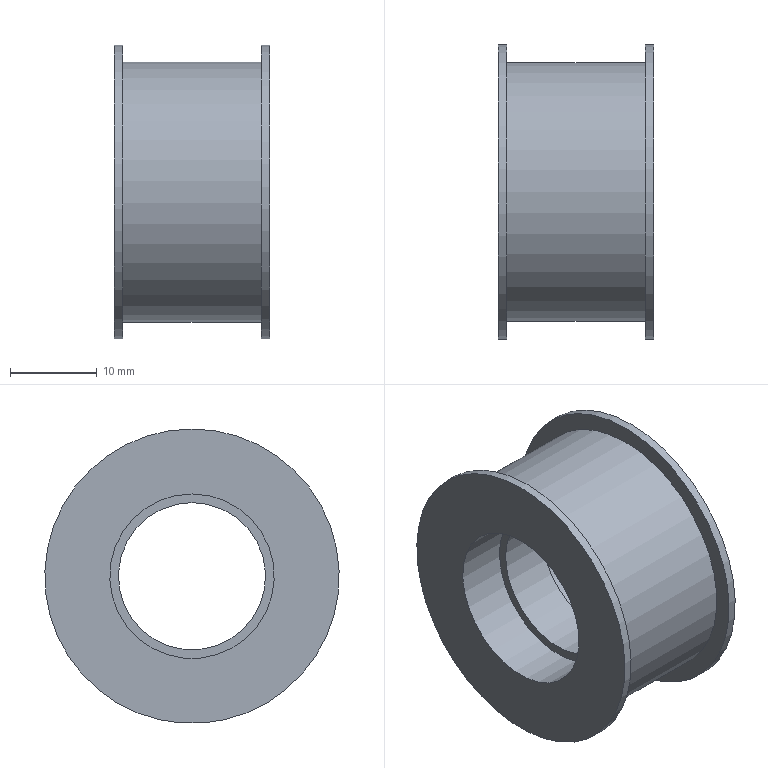Part | NX | 1 solid | 12 faces | box 18 x 34 x 34 mm | volume 8361 mm3 | cylinder 6 | plane 6 | commonest cylinder face diameters 19 x2 34 x2 17 x1 30 x1
STEP:
#1=CARTESIAN_POINT('',(-9.,0.,17.));
#2=VERTEX_POINT('',#1);
#3=CARTESIAN_POINT('',(-9.,0.,0.));
#4=DIRECTION('',(-1.,0.,0.));
#5=DIRECTION('',(0.,0.,1.));
#6=AXIS2_PLACEMENT_3D('',#3,#4,#5);
#7=CIRCLE('',#6,17.);
#8=EDGE_CURVE('',#2,#2,#7,.T.);
#9=ORIENTED_EDGE('',*,*,#8,.F.);
#10=EDGE_LOOP('',(#9));
#11=FACE_BOUND('',#10,.T.);
#12=CARTESIAN_POINT('',(-8.,0.,17.));
#13=VERTEX_POINT('',#12);
#14=CARTESIAN_POINT('',(-8.,0.,0.));
#15=DIRECTION('',(-1.,0.,0.));
#16=DIRECTION('',(0.,0.,1.));
#17=AXIS2_PLACEMENT_3D('',#14,#15,#16);
#18=CIRCLE('',#17,17.);
#19=EDGE_CURVE('',#13,#13,#18,.T.);
#20=ORIENTED_EDGE('',*,*,#19,.T.);
#21=EDGE_LOOP('',(#20));
#22=FACE_BOUND('',#21,.T.);
#23=CARTESIAN_POINT('',(9.,0.,0.));
#24=DIRECTION('',(-1.,0.,0.));
#25=DIRECTION('',(0.,0.,1.));
#26=AXIS2_PLACEMENT_3D('',#23,#24,#25);
#27=CYLINDRICAL_SURFACE('',#26,17.);
#28=ADVANCED_FACE('',(#11,#22),#27,.T.);
#29=CARTESIAN_POINT('',(-9.,0.,9.5));
#30=VERTEX_POINT('',#29);
#31=CARTESIAN_POINT('',(-9.,0.,0.));
#32=DIRECTION('',(-1.,0.,0.));
#33=DIRECTION('',(0.,0.,1.));
#34=AXIS2_PLACEMENT_3D('',#31,#32,#33);
#35=CIRCLE('',#34,9.5);
#36=EDGE_CURVE('',#30,#30,#35,.T.);
#37=ORIENTED_EDGE('',*,*,#36,.F.);
#38=EDGE_LOOP('',(#37));
#39=FACE_BOUND('',#38,.T.);
#40=ORIENTED_EDGE('',*,*,#8,.T.);
#41=EDGE_LOOP('',(#40));
#42=FACE_BOUND('',#41,.T.);
#43=CARTESIAN_POINT('',(-9.,17.,0.));
#44=DIRECTION('',(1.,0.,0.));
#45=DIRECTION('',(0.,0.,-1.));
#46=AXIS2_PLACEMENT_3D('',#43,#44,#45);
#47=PLANE('',#46);
#48=ADVANCED_FACE('',(#39,#42),#47,.F.);
#49=CARTESIAN_POINT('',(-3.,0.,9.5));
#50=VERTEX_POINT('',#49);
#51=CARTESIAN_POINT('',(-3.,0.,0.));
#52=DIRECTION('',(-1.,0.,0.));
#53=DIRECTION('',(0.,0.,1.));
#54=AXIS2_PLACEMENT_3D('',#51,#52,#53);
#55=CIRCLE('',#54,9.5);
#56=EDGE_CURVE('',#50,#50,#55,.T.);
#57=ORIENTED_EDGE('',*,*,#56,.F.);
#58=EDGE_LOOP('',(#57));
#59=FACE_BOUND('',#58,.T.);
#60=ORIENTED_EDGE('',*,*,#36,.T.);
#61=EDGE_LOOP('',(#60));
#62=FACE_BOUND('',#61,.T.);
#63=CARTESIAN_POINT('',(9.,0.,0.));
#64=DIRECTION('',(-1.,0.,0.));
#65=DIRECTION('',(0.,0.,1.));
#66=AXIS2_PLACEMENT_3D('',#63,#64,#65);
#67=CYLINDRICAL_SURFACE('',#66,9.5);
#68=ADVANCED_FACE('',(#59,#62),#67,.F.);
#69=CARTESIAN_POINT('',(-3.,0.,8.5));
#70=VERTEX_POINT('',#69);
#71=CARTESIAN_POINT('',(-3.,0.,0.));
#72=DIRECTION('',(-1.,0.,0.));
#73=DIRECTION('',(0.,0.,1.));
#74=AXIS2_PLACEMENT_3D('',#71,#72,#73);
#75=CIRCLE('',#74,8.5);
#76=EDGE_CURVE('',#70,#70,#75,.T.);
#77=ORIENTED_EDGE('',*,*,#76,.F.);
#78=EDGE_LOOP('',(#77));
#79=FACE_BOUND('',#78,.T.);
#80=ORIENTED_EDGE('',*,*,#56,.T.);
#81=EDGE_LOOP('',(#80));
#82=FACE_BOUND('',#81,.T.);
#83=CARTESIAN_POINT('',(-3.,9.5,0.));
#84=DIRECTION('',(1.,0.,0.));
#85=DIRECTION('',(0.,0.,-1.));
#86=AXIS2_PLACEMENT_3D('',#83,#84,#85);
#87=PLANE('',#86);
#88=ADVANCED_FACE('',(#79,#82),#87,.F.);
#89=CARTESIAN_POINT('',(3.,0.,8.5));
#90=VERTEX_POINT('',#89);
#91=CARTESIAN_POINT('',(3.,0.,0.));
#92=DIRECTION('',(-1.,0.,0.));
#93=DIRECTION('',(0.,0.,1.));
#94=AXIS2_PLACEMENT_3D('',#91,#92,#93);
#95=CIRCLE('',#94,8.5);
#96=EDGE_CURVE('',#90,#90,#95,.T.);
#97=ORIENTED_EDGE('',*,*,#96,.F.);
#98=EDGE_LOOP('',(#97));
#99=FACE_BOUND('',#98,.T.);
#100=ORIENTED_EDGE('',*,*,#76,.T.);
#101=EDGE_LOOP('',(#100));
#102=FACE_BOUND('',#101,.T.);
#103=CARTESIAN_POINT('',(9.,0.,0.));
#104=DIRECTION('',(-1.,0.,0.));
#105=DIRECTION('',(0.,0.,1.));
#106=AXIS2_PLACEMENT_3D('',#103,#104,#105);
#107=CYLINDRICAL_SURFACE('',#106,8.5);
#108=ADVANCED_FACE('',(#99,#102),#107,.F.);
#109=CARTESIAN_POINT('',(3.,0.,9.5));
#110=VERTEX_POINT('',#109);
#111=CARTESIAN_POINT('',(3.,0.,0.));
#112=DIRECTION('',(-1.,0.,0.));
#113=DIRECTION('',(0.,0.,1.));
#114=AXIS2_PLACEMENT_3D('',#111,#112,#113);
#115=CIRCLE('',#114,9.5);
#116=EDGE_CURVE('',#110,#110,#115,.T.);
#117=ORIENTED_EDGE('',*,*,#116,.F.);
#118=EDGE_LOOP('',(#117));
#119=FACE_BOUND('',#118,.T.);
#120=ORIENTED_EDGE('',*,*,#96,.T.);
#121=EDGE_LOOP('',(#120));
#122=FACE_BOUND('',#121,.T.);
#123=CARTESIAN_POINT('',(3.,8.5,0.));
#124=DIRECTION('',(-1.,0.,0.));
#125=DIRECTION('',(0.,0.,1.));
#126=AXIS2_PLACEMENT_3D('',#123,#124,#125);
#127=PLANE('',#126);
#128=ADVANCED_FACE('',(#119,#122),#127,.F.);
#129=CARTESIAN_POINT('',(9.,0.,9.5));
#130=VERTEX_POINT('',#129);
#131=CARTESIAN_POINT('',(9.,0.,0.));
#132=DIRECTION('',(-1.,0.,0.));
#133=DIRECTION('',(0.,0.,1.));
#134=AXIS2_PLACEMENT_3D('',#131,#132,#133);
#135=CIRCLE('',#134,9.5);
#136=EDGE_CURVE('',#130,#130,#135,.T.);
#137=ORIENTED_EDGE('',*,*,#136,.F.);
#138=EDGE_LOOP('',(#137));
#139=FACE_BOUND('',#138,.T.);
#140=ORIENTED_EDGE('',*,*,#116,.T.);
#141=EDGE_LOOP('',(#140));
#142=FACE_BOUND('',#141,.T.);
#143=CARTESIAN_POINT('',(9.,0.,0.));
#144=DIRECTION('',(-1.,0.,0.));
#145=DIRECTION('',(0.,0.,1.));
#146=AXIS2_PLACEMENT_3D('',#143,#144,#145);
#147=CYLINDRICAL_SURFACE('',#146,9.5);
#148=ADVANCED_FACE('',(#139,#142),#147,.F.);
#149=CARTESIAN_POINT('',(9.,0.,17.));
#150=VERTEX_POINT('',#149);
#151=CARTESIAN_POINT('',(9.,0.,0.));
#152=DIRECTION('',(-1.,0.,0.));
#153=DIRECTION('',(0.,0.,1.));
#154=AXIS2_PLACEMENT_3D('',#151,#152,#153);
#155=CIRCLE('',#154,17.);
#156=EDGE_CURVE('',#150,#150,#155,.T.);
#157=ORIENTED_EDGE('',*,*,#156,.F.);
#158=EDGE_LOOP('',(#157));
#159=FACE_BOUND('',#158,.T.);
#160=ORIENTED_EDGE('',*,*,#136,.T.);
#161=EDGE_LOOP('',(#160));
#162=FACE_BOUND('',#161,.T.);
#163=CARTESIAN_POINT('',(9.,9.5,0.));
#164=DIRECTION('',(-1.,0.,0.));
#165=DIRECTION('',(0.,0.,1.));
#166=AXIS2_PLACEMENT_3D('',#163,#164,#165);
#167=PLANE('',#166);
#168=ADVANCED_FACE('',(#159,#162),#167,.F.);
#169=CARTESIAN_POINT('',(8.,0.,17.));
#170=VERTEX_POINT('',#169);
#171=CARTESIAN_POINT('',(8.,0.,0.));
#172=DIRECTION('',(-1.,0.,0.));
#173=DIRECTION('',(0.,0.,1.));
#174=AXIS2_PLACEMENT_3D('',#171,#172,#173);
#175=CIRCLE('',#174,17.);
#176=EDGE_CURVE('',#170,#170,#175,.T.);
#177=ORIENTED_EDGE('',*,*,#176,.F.);
#178=EDGE_LOOP('',(#177));
#179=FACE_BOUND('',#178,.T.);
#180=ORIENTED_EDGE('',*,*,#156,.T.);
#181=EDGE_LOOP('',(#180));
#182=FACE_BOUND('',#181,.T.);
#183=CARTESIAN_POINT('',(9.,0.,0.));
#184=DIRECTION('',(-1.,0.,0.));
#185=DIRECTION('',(0.,0.,1.));
#186=AXIS2_PLACEMENT_3D('',#183,#184,#185);
#187=CYLINDRICAL_SURFACE('',#186,17.);
#188=ADVANCED_FACE('',(#179,#182),#187,.T.);
#189=CARTESIAN_POINT('',(8.,0.,15.));
#190=VERTEX_POINT('',#189);
#191=CARTESIAN_POINT('',(8.,0.,0.));
#192=DIRECTION('',(-1.,0.,0.));
#193=DIRECTION('',(0.,0.,1.));
#194=AXIS2_PLACEMENT_3D('',#191,#192,#193);
#195=CIRCLE('',#194,15.);
#196=EDGE_CURVE('',#190,#190,#195,.T.);
#197=ORIENTED_EDGE('',*,*,#196,.F.);
#198=EDGE_LOOP('',(#197));
#199=FACE_BOUND('',#198,.T.);
#200=ORIENTED_EDGE('',*,*,#176,.T.);
#201=EDGE_LOOP('',(#200));
#202=FACE_BOUND('',#201,.T.);
#203=CARTESIAN_POINT('',(8.,17.,0.));
#204=DIRECTION('',(1.,0.,0.));
#205=DIRECTION('',(0.,0.,-1.));
#206=AXIS2_PLACEMENT_3D('',#203,#204,#205);
#207=PLANE('',#206);
#208=ADVANCED_FACE('',(#199,#202),#207,.F.);
#209=CARTESIAN_POINT('',(-8.,0.,15.));
#210=VERTEX_POINT('',#209);
#211=CARTESIAN_POINT('',(-8.,0.,0.));
#212=DIRECTION('',(-1.,0.,0.));
#213=DIRECTION('',(0.,0.,1.));
#214=AXIS2_PLACEMENT_3D('',#211,#212,#213);
#215=CIRCLE('',#214,15.);
#216=EDGE_CURVE('',#210,#210,#215,.T.);
#217=ORIENTED_EDGE('',*,*,#216,.F.);
#218=EDGE_LOOP('',(#217));
#219=FACE_BOUND('',#218,.T.);
#220=ORIENTED_EDGE('',*,*,#196,.T.);
#221=EDGE_LOOP('',(#220));
#222=FACE_BOUND('',#221,.T.);
#223=CARTESIAN_POINT('',(9.,0.,0.));
#224=DIRECTION('',(-1.,0.,0.));
#225=DIRECTION('',(0.,0.,1.));
#226=AXIS2_PLACEMENT_3D('',#223,#224,#225);
#227=CYLINDRICAL_SURFACE('',#226,15.);
#228=ADVANCED_FACE('',(#219,#222),#227,.T.);
#229=ORIENTED_EDGE('',*,*,#19,.F.);
#230=EDGE_LOOP('',(#229));
#231=FACE_BOUND('',#230,.T.);
#232=ORIENTED_EDGE('',*,*,#216,.T.);
#233=EDGE_LOOP('',(#232));
#234=FACE_BOUND('',#233,.T.);
#235=CARTESIAN_POINT('',(-8.,15.,0.));
#236=DIRECTION('',(-1.,0.,0.));
#237=DIRECTION('',(0.,0.,1.));
#238=AXIS2_PLACEMENT_3D('',#235,#236,#237);
#239=PLANE('',#238);
#240=ADVANCED_FACE('',(#231,#234),#239,.F.);
#241=CLOSED_SHELL('',(#28,#48,#68,#88,#108,#128,#148,#168,#188,#208,#228,#240));
#242=MANIFOLD_SOLID_BREP('',#241);
#243=(LENGTH_UNIT()NAMED_UNIT(*)SI_UNIT(.MILLI.,.METRE.));
#244=UNCERTAINTY_MEASURE_WITH_UNIT(LENGTH_MEASURE(0.00001),#243,'','');
#245=(NAMED_UNIT(*)PLANE_ANGLE_UNIT()SI_UNIT($,.RADIAN.));
#246=(NAMED_UNIT(*)SI_UNIT($,.STERADIAN.)SOLID_ANGLE_UNIT());
#247=(GEOMETRIC_REPRESENTATION_CONTEXT(3)GLOBAL_UNCERTAINTY_ASSIGNED_CONTEXT((#244))GLOBAL_UNIT_ASSIGNED_CONTEXT((#243,#245,#246))REPRESENTATION_CONTEXT('',''));
#248=ADVANCED_BREP_SHAPE_REPRESENTATION('',(#242),#247);